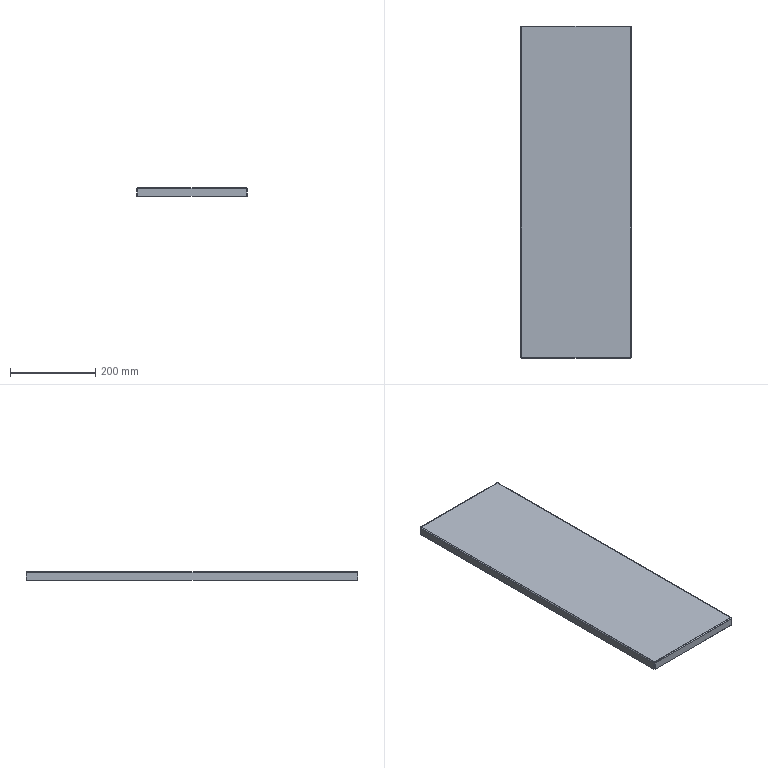Part | STEP file | X77-03020 | 1 solid | 38 faces | box 258 x 778 x 20 mm | volume 356098 mm3 | plane 22 | spline 8 | cylinder 8 | commonest cylinder face diameters 1.473 x4 4.473 x4